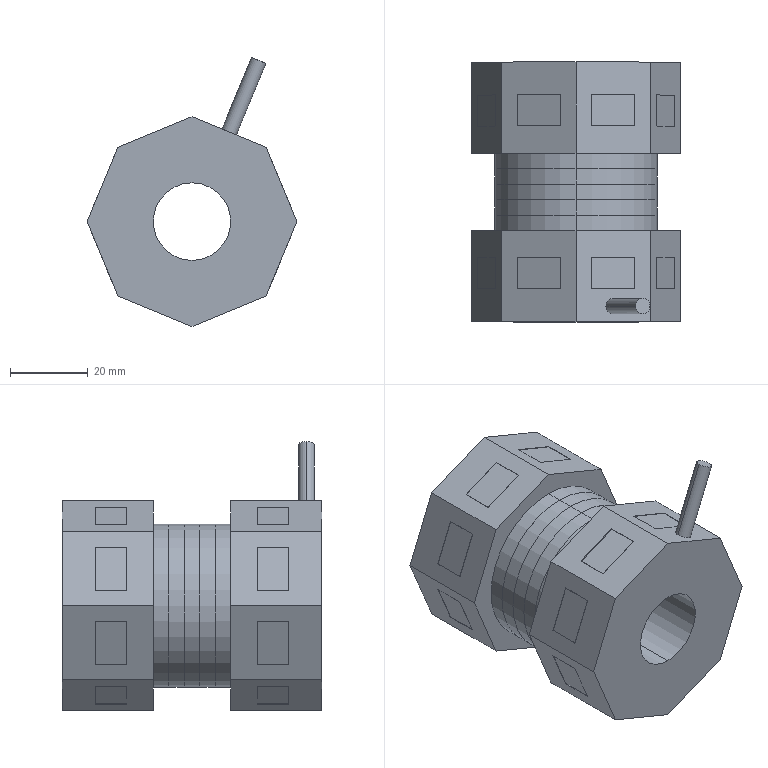Part | SolidWorks | features ICE 6, CirPattern 1, Extrusion 1, HoleWzd 1, MirrorPattern 1, RefAxis 1, Revolution 1 | 1 solid | 135 faces | box 54.12 x 67 x 69.4 mm | volume 103995 mm3 | plane 105 | cylinder 22 | cone 8 | commonest cylinder face diameters 3.3 x8 42 x4 42.01 x4 4 x2 20 x2 42.02 x2